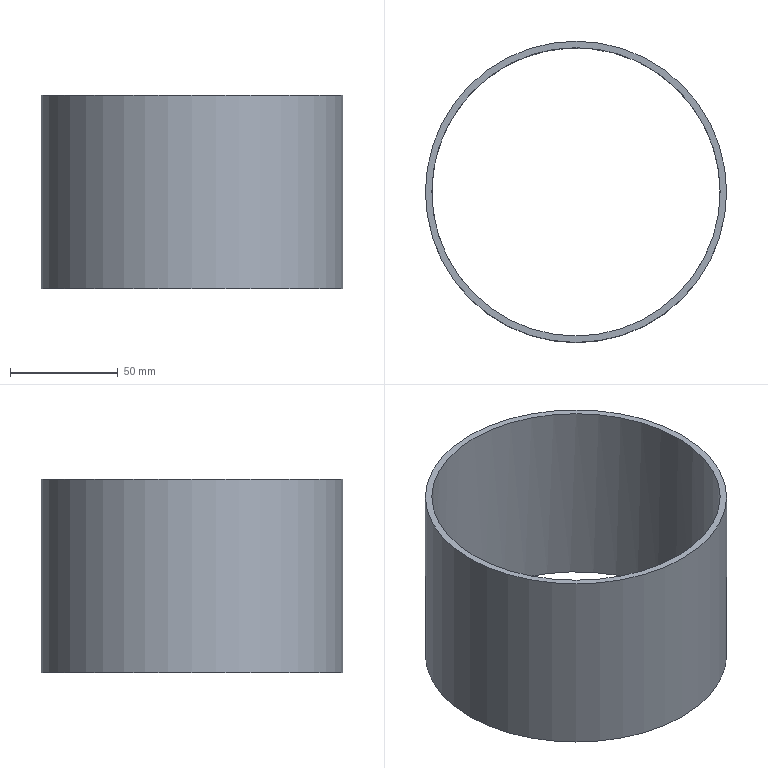Part | NX | features solid 2 | 1 solid | 4 faces | box 140 x 140 x 90 mm | volume 116208 mm3 | plane 2 | cylinder 2 | commonest cylinder face diameters 134 x1 140 x1
STEP:
#1=CARTESIAN_POINT('',(-1532.452,860.96,-40.));
#2=VERTEX_POINT('',#1);
#3=CARTESIAN_POINT('',(-1465.452,860.96,-40.));
#4=DIRECTION('',(0.,0.,1.));
#5=DIRECTION('',(-1.,0.,0.));
#6=AXIS2_PLACEMENT_3D('',#3,#4,#5);
#7=CIRCLE('',#6,67.);
#8=EDGE_CURVE('',#2,#2,#7,.F.);
#9=ORIENTED_EDGE('',*,*,#8,.T.);
#10=EDGE_LOOP('',(#9));
#11=FACE_BOUND('',#10,.T.);
#12=CARTESIAN_POINT('',(-1535.452,860.96,-40.));
#13=VERTEX_POINT('',#12);
#14=CARTESIAN_POINT('',(-1465.452,860.96,-40.));
#15=DIRECTION('',(0.,0.,1.));
#16=DIRECTION('',(-1.,0.,0.));
#17=AXIS2_PLACEMENT_3D('',#14,#15,#16);
#18=CIRCLE('',#17,70.);
#19=EDGE_CURVE('',#13,#13,#18,.F.);
#20=ORIENTED_EDGE('',*,*,#19,.F.);
#21=EDGE_LOOP('',(#20));
#22=FACE_BOUND('',#21,.T.);
#23=CARTESIAN_POINT('',(-1465.452,860.96,-40.));
#24=DIRECTION('',(0.,0.,-1.));
#25=DIRECTION('',(-0.7071,0.7071,0.));
#26=AXIS2_PLACEMENT_3D('',#23,#24,#25);
#27=PLANE('',#26);
#28=ADVANCED_FACE('',(#11,#22),#27,.F.);
#29=CARTESIAN_POINT('',(-1418.075,813.584,-130.));
#30=VERTEX_POINT('',#29);
#31=CARTESIAN_POINT('',(-1465.452,860.96,-130.));
#32=DIRECTION('',(0.,0.,-1.));
#33=DIRECTION('',(0.7071,-0.7071,0.));
#34=AXIS2_PLACEMENT_3D('',#31,#32,#33);
#35=CIRCLE('',#34,67.);
#36=EDGE_CURVE('',#30,#30,#35,.T.);
#37=ORIENTED_EDGE('',*,*,#36,.F.);
#38=EDGE_LOOP('',(#37));
#39=FACE_BOUND('',#38,.T.);
#40=CARTESIAN_POINT('',(-1415.954,811.462,-130.));
#41=VERTEX_POINT('',#40);
#42=CARTESIAN_POINT('',(-1465.452,860.96,-130.));
#43=DIRECTION('',(0.,0.,-1.));
#44=DIRECTION('',(0.7071,-0.7071,0.));
#45=AXIS2_PLACEMENT_3D('',#42,#43,#44);
#46=CIRCLE('',#45,70.);
#47=EDGE_CURVE('',#41,#41,#46,.T.);
#48=ORIENTED_EDGE('',*,*,#47,.T.);
#49=EDGE_LOOP('',(#48));
#50=FACE_BOUND('',#49,.T.);
#51=CARTESIAN_POINT('',(-1465.452,860.96,-130.));
#52=DIRECTION('',(0.,0.,-1.));
#53=DIRECTION('',(-0.7071,0.7071,0.));
#54=AXIS2_PLACEMENT_3D('',#51,#52,#53);
#55=PLANE('',#54);
#56=ADVANCED_FACE('',(#39,#50),#55,.T.);
#57=ORIENTED_EDGE('',*,*,#8,.F.);
#58=EDGE_LOOP('',(#57));
#59=FACE_BOUND('',#58,.T.);
#60=ORIENTED_EDGE('',*,*,#36,.T.);
#61=EDGE_LOOP('',(#60));
#62=FACE_BOUND('',#61,.T.);
#63=CARTESIAN_POINT('',(-1465.452,860.96,-130.));
#64=DIRECTION('',(0.,0.,1.));
#65=DIRECTION('',(0.7071,-0.7071,0.));
#66=AXIS2_PLACEMENT_3D('',#63,#64,#65);
#67=CYLINDRICAL_SURFACE('',#66,67.);
#68=ADVANCED_FACE('',(#59,#62),#67,.F.);
#69=ORIENTED_EDGE('',*,*,#19,.T.);
#70=EDGE_LOOP('',(#69));
#71=FACE_BOUND('',#70,.T.);
#72=ORIENTED_EDGE('',*,*,#47,.F.);
#73=EDGE_LOOP('',(#72));
#74=FACE_BOUND('',#73,.T.);
#75=CARTESIAN_POINT('',(-1465.452,860.96,-130.));
#76=DIRECTION('',(0.,0.,1.));
#77=DIRECTION('',(0.7071,-0.7071,0.));
#78=AXIS2_PLACEMENT_3D('',#75,#76,#77);
#79=CYLINDRICAL_SURFACE('',#78,70.);
#80=ADVANCED_FACE('',(#71,#74),#79,.T.);
#81=CLOSED_SHELL('',(#28,#56,#68,#80));
#82=MANIFOLD_SOLID_BREP('',#81);
#83=(LENGTH_UNIT()NAMED_UNIT(*)SI_UNIT(.MILLI.,.METRE.));
#84=UNCERTAINTY_MEASURE_WITH_UNIT(LENGTH_MEASURE(0.00001),#83,'','');
#85=(NAMED_UNIT(*)PLANE_ANGLE_UNIT()SI_UNIT($,.RADIAN.));
#86=(NAMED_UNIT(*)SI_UNIT($,.STERADIAN.)SOLID_ANGLE_UNIT());
#87=(GEOMETRIC_REPRESENTATION_CONTEXT(3)GLOBAL_UNCERTAINTY_ASSIGNED_CONTEXT((#84))GLOBAL_UNIT_ASSIGNED_CONTEXT((#83,#85,#86))REPRESENTATION_CONTEXT('',''));
#88=ADVANCED_BREP_SHAPE_REPRESENTATION('',(#82),#87);